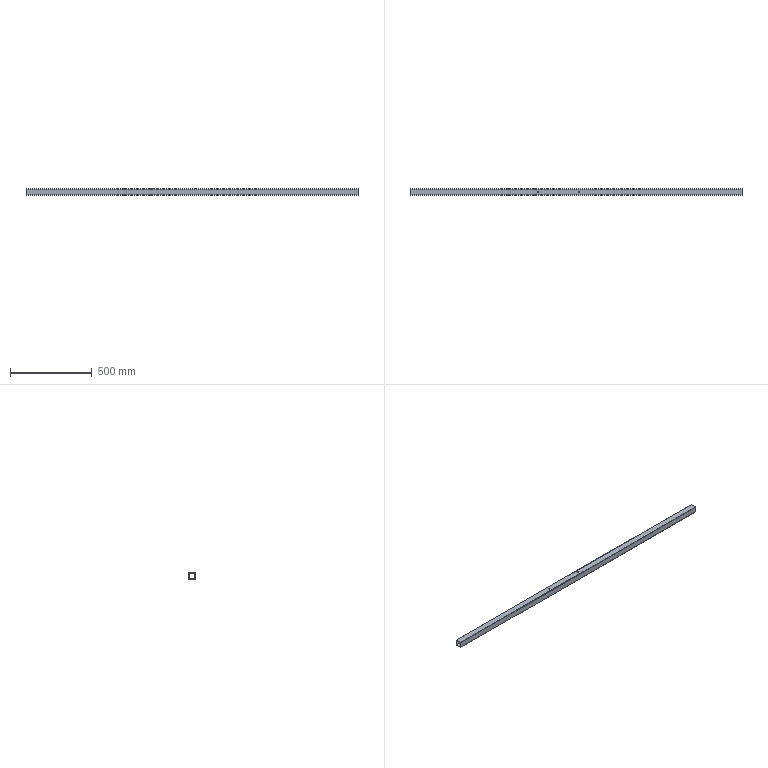Part | NX | features BREP 1 | 1 solid | 18 faces | box 2032 x 38.1 x 38.1 mm | volume 548857 mm3 | plane 10 | cylinder 8 | commonest cylinder face diameters 3.175 x4 5.842 x4
STEP:
#1=CARTESIAN_POINT('',(-1016.,19.05,-17.462));
#2=VERTEX_POINT('',#1);
#3=CARTESIAN_POINT('',(-1016.,19.05,17.462));
#4=VERTEX_POINT('',#3);
#5=CARTESIAN_POINT('',(-1016.,19.05,-17.462));
#6=DIRECTION('',(0.,0.,1.));
#7=VECTOR('',#6,1000.);
#8=LINE('',#5,#7);
#9=EDGE_CURVE('',#2,#4,#8,.T.);
#10=ORIENTED_EDGE('',*,*,#9,.F.);
#11=CARTESIAN_POINT('',(-1016.,17.462,-19.05));
#12=VERTEX_POINT('',#11);
#13=CARTESIAN_POINT('',(-1016.,17.462,-17.462));
#14=DIRECTION('',(-1.,0.,0.));
#15=DIRECTION('',(0.,1.,0.));
#16=AXIS2_PLACEMENT_3D('',#13,#14,#15);
#17=CIRCLE('',#16,1.587);
#18=EDGE_CURVE('',#2,#12,#17,.T.);
#19=ORIENTED_EDGE('',*,*,#18,.T.);
#20=CARTESIAN_POINT('',(-1016.,-17.462,-19.05));
#21=VERTEX_POINT('',#20);
#22=CARTESIAN_POINT('',(-1016.,-17.462,-19.05));
#23=DIRECTION('',(0.,1.,0.));
#24=VECTOR('',#23,1000.);
#25=LINE('',#22,#24);
#26=EDGE_CURVE('',#21,#12,#25,.T.);
#27=ORIENTED_EDGE('',*,*,#26,.F.);
#28=CARTESIAN_POINT('',(-1016.,-19.05,-17.462));
#29=VERTEX_POINT('',#28);
#30=CARTESIAN_POINT('',(-1016.,-17.462,-17.462));
#31=DIRECTION('',(-1.,0.,0.));
#32=DIRECTION('',(0.,0.,-1.));
#33=AXIS2_PLACEMENT_3D('',#30,#31,#32);
#34=CIRCLE('',#33,1.587);
#35=EDGE_CURVE('',#21,#29,#34,.T.);
#36=ORIENTED_EDGE('',*,*,#35,.T.);
#37=CARTESIAN_POINT('',(-1016.,-19.05,17.462));
#38=VERTEX_POINT('',#37);
#39=CARTESIAN_POINT('',(-1016.,-19.05,17.462));
#40=DIRECTION('',(0.,0.,-1.));
#41=VECTOR('',#40,1000.);
#42=LINE('',#39,#41);
#43=EDGE_CURVE('',#38,#29,#42,.T.);
#44=ORIENTED_EDGE('',*,*,#43,.F.);
#45=CARTESIAN_POINT('',(-1016.,-17.462,19.05));
#46=VERTEX_POINT('',#45);
#47=CARTESIAN_POINT('',(-1016.,-17.462,17.462));
#48=DIRECTION('',(-1.,0.,0.));
#49=DIRECTION('',(0.,-1.,0.));
#50=AXIS2_PLACEMENT_3D('',#47,#48,#49);
#51=CIRCLE('',#50,1.587);
#52=EDGE_CURVE('',#38,#46,#51,.T.);
#53=ORIENTED_EDGE('',*,*,#52,.T.);
#54=CARTESIAN_POINT('',(-1016.,17.462,19.05));
#55=VERTEX_POINT('',#54);
#56=CARTESIAN_POINT('',(-1016.,17.462,19.05));
#57=DIRECTION('',(0.,-1.,0.));
#58=VECTOR('',#57,1000.);
#59=LINE('',#56,#58);
#60=EDGE_CURVE('',#55,#46,#59,.T.);
#61=ORIENTED_EDGE('',*,*,#60,.F.);
#62=CARTESIAN_POINT('',(-1016.,17.462,17.462));
#63=DIRECTION('',(-1.,0.,0.));
#64=DIRECTION('',(0.,0.,1.));
#65=AXIS2_PLACEMENT_3D('',#62,#63,#64);
#66=CIRCLE('',#65,1.587);
#67=EDGE_CURVE('',#55,#4,#66,.T.);
#68=ORIENTED_EDGE('',*,*,#67,.T.);
#69=EDGE_LOOP('',(#10,#19,#27,#36,#44,#53,#61,#68));
#70=FACE_BOUND('',#69,.T.);
#71=CARTESIAN_POINT('',(-1016.,17.17,17.17));
#72=VERTEX_POINT('',#71);
#73=CARTESIAN_POINT('',(-1016.,17.17,-17.17));
#74=VERTEX_POINT('',#73);
#75=CARTESIAN_POINT('',(-1016.,17.17,17.17));
#76=DIRECTION('',(0.,0.,-1.));
#77=VECTOR('',#76,1000.);
#78=LINE('',#75,#77);
#79=EDGE_CURVE('',#72,#74,#78,.T.);
#80=ORIENTED_EDGE('',*,*,#79,.F.);
#81=CARTESIAN_POINT('',(-1016.,-17.17,17.17));
#82=VERTEX_POINT('',#81);
#83=CARTESIAN_POINT('',(-1016.,-17.17,17.17));
#84=DIRECTION('',(0.,1.,0.));
#85=VECTOR('',#84,1000.);
#86=LINE('',#83,#85);
#87=EDGE_CURVE('',#82,#72,#86,.T.);
#88=ORIENTED_EDGE('',*,*,#87,.F.);
#89=CARTESIAN_POINT('',(-1016.,-17.17,-17.17));
#90=VERTEX_POINT('',#89);
#91=CARTESIAN_POINT('',(-1016.,-17.17,-17.17));
#92=DIRECTION('',(0.,0.,1.));
#93=VECTOR('',#92,1000.);
#94=LINE('',#91,#93);
#95=EDGE_CURVE('',#90,#82,#94,.T.);
#96=ORIENTED_EDGE('',*,*,#95,.F.);
#97=CARTESIAN_POINT('',(-1016.,17.17,-17.17));
#98=DIRECTION('',(0.,-1.,0.));
#99=VECTOR('',#98,1000.);
#100=LINE('',#97,#99);
#101=EDGE_CURVE('',#74,#90,#100,.T.);
#102=ORIENTED_EDGE('',*,*,#101,.F.);
#103=EDGE_LOOP('',(#80,#88,#96,#102));
#104=FACE_BOUND('',#103,.T.);
#105=CARTESIAN_POINT('',(-1016.,0.,0.));
#106=DIRECTION('',(1.,0.,0.));
#107=DIRECTION('',(0.,1.,0.));
#108=AXIS2_PLACEMENT_3D('',#105,#106,#107);
#109=PLANE('',#108);
#110=ADVANCED_FACE('',(#70,#104),#109,.F.);
#111=CARTESIAN_POINT('',(1016.,-17.17,-17.17));
#112=VERTEX_POINT('',#111);
#113=CARTESIAN_POINT('',(-1016.,-17.17,-17.17));
#114=DIRECTION('',(1.,0.,0.));
#115=VECTOR('',#114,1000.);
#116=LINE('',#113,#115);
#117=EDGE_CURVE('',#90,#112,#116,.T.);
#118=ORIENTED_EDGE('',*,*,#117,.T.);
#119=CARTESIAN_POINT('',(1016.,17.17,-17.17));
#120=VERTEX_POINT('',#119);
#121=CARTESIAN_POINT('',(1016.,17.17,-17.17));
#122=DIRECTION('',(0.,-1.,0.));
#123=VECTOR('',#122,1000.);
#124=LINE('',#121,#123);
#125=EDGE_CURVE('',#120,#112,#124,.T.);
#126=ORIENTED_EDGE('',*,*,#125,.F.);
#127=CARTESIAN_POINT('',(-1016.,17.17,-17.17));
#128=DIRECTION('',(1.,0.,0.));
#129=VECTOR('',#128,1000.);
#130=LINE('',#127,#129);
#131=EDGE_CURVE('',#74,#120,#130,.T.);
#132=ORIENTED_EDGE('',*,*,#131,.F.);
#133=ORIENTED_EDGE('',*,*,#101,.T.);
#134=EDGE_LOOP('',(#118,#126,#132,#133));
#135=FACE_BOUND('',#134,.T.);
#136=CARTESIAN_POINT('',(-1016.,17.17,-17.17));
#137=DIRECTION('',(0.,0.,1.));
#138=DIRECTION('',(1.,0.,0.));
#139=AXIS2_PLACEMENT_3D('',#136,#137,#138);
#140=PLANE('',#139);
#141=ADVANCED_FACE('',(#135),#140,.T.);
#142=ORIENTED_EDGE('',*,*,#131,.T.);
#143=CARTESIAN_POINT('',(1016.,17.17,17.17));
#144=VERTEX_POINT('',#143);
#145=CARTESIAN_POINT('',(1016.,17.17,17.17));
#146=DIRECTION('',(0.,0.,-1.));
#147=VECTOR('',#146,1000.);
#148=LINE('',#145,#147);
#149=EDGE_CURVE('',#144,#120,#148,.T.);
#150=ORIENTED_EDGE('',*,*,#149,.F.);
#151=CARTESIAN_POINT('',(-1016.,17.17,17.17));
#152=DIRECTION('',(1.,0.,0.));
#153=VECTOR('',#152,1000.);
#154=LINE('',#151,#153);
#155=EDGE_CURVE('',#72,#144,#154,.T.);
#156=ORIENTED_EDGE('',*,*,#155,.F.);
#157=ORIENTED_EDGE('',*,*,#79,.T.);
#158=EDGE_LOOP('',(#142,#150,#156,#157));
#159=FACE_BOUND('',#158,.T.);
#160=CARTESIAN_POINT('',(-1016.,17.17,17.17));
#161=DIRECTION('',(0.,-1.,0.));
#162=DIRECTION('',(0.,0.,-1.));
#163=AXIS2_PLACEMENT_3D('',#160,#161,#162);
#164=PLANE('',#163);
#165=ADVANCED_FACE('',(#159),#164,.T.);
#166=ORIENTED_EDGE('',*,*,#155,.T.);
#167=CARTESIAN_POINT('',(1016.,-17.17,17.17));
#168=VERTEX_POINT('',#167);
#169=CARTESIAN_POINT('',(1016.,-17.17,17.17));
#170=DIRECTION('',(0.,1.,0.));
#171=VECTOR('',#170,1000.);
#172=LINE('',#169,#171);
#173=EDGE_CURVE('',#168,#144,#172,.T.);
#174=ORIENTED_EDGE('',*,*,#173,.F.);
#175=CARTESIAN_POINT('',(-1016.,-17.17,17.17));
#176=DIRECTION('',(1.,0.,0.));
#177=VECTOR('',#176,1000.);
#178=LINE('',#175,#177);
#179=EDGE_CURVE('',#82,#168,#178,.T.);
#180=ORIENTED_EDGE('',*,*,#179,.F.);
#181=ORIENTED_EDGE('',*,*,#87,.T.);
#182=EDGE_LOOP('',(#166,#174,#180,#181));
#183=FACE_BOUND('',#182,.T.);
#184=CARTESIAN_POINT('',(17.907,0.,17.17));
#185=VERTEX_POINT('',#184);
#186=CARTESIAN_POINT('',(23.749,0.,17.17));
#187=VERTEX_POINT('',#186);
#188=CARTESIAN_POINT('',(20.828,0.,17.17));
#189=DIRECTION('',(0.,0.,1.));
#190=DIRECTION('',(-1.,0.,0.));
#191=AXIS2_PLACEMENT_3D('',#188,#189,#190);
#192=CIRCLE('',#191,2.921);
#193=EDGE_CURVE('',#185,#187,#192,.T.);
#194=ORIENTED_EDGE('',*,*,#193,.T.);
#195=CARTESIAN_POINT('',(20.828,0.,17.17));
#196=DIRECTION('',(0.,0.,1.));
#197=DIRECTION('',(1.,0.,0.));
#198=AXIS2_PLACEMENT_3D('',#195,#196,#197);
#199=CIRCLE('',#198,2.921);
#200=EDGE_CURVE('',#187,#185,#199,.T.);
#201=ORIENTED_EDGE('',*,*,#200,.T.);
#202=EDGE_LOOP('',(#194,#201));
#203=FACE_BOUND('',#202,.T.);
#204=CARTESIAN_POINT('',(-233.553,0.,17.17));
#205=VERTEX_POINT('',#204);
#206=CARTESIAN_POINT('',(-227.711,0.,17.17));
#207=VERTEX_POINT('',#206);
#208=CARTESIAN_POINT('',(-230.632,0.,17.17));
#209=DIRECTION('',(0.,0.,1.));
#210=DIRECTION('',(-1.,0.,0.));
#211=AXIS2_PLACEMENT_3D('',#208,#209,#210);
#212=CIRCLE('',#211,2.921);
#213=EDGE_CURVE('',#205,#207,#212,.T.);
#214=ORIENTED_EDGE('',*,*,#213,.T.);
#215=CARTESIAN_POINT('',(-230.632,0.,17.17));
#216=DIRECTION('',(0.,0.,1.));
#217=DIRECTION('',(1.,0.,0.));
#218=AXIS2_PLACEMENT_3D('',#215,#216,#217);
#219=CIRCLE('',#218,2.921);
#220=EDGE_CURVE('',#207,#205,#219,.T.);
#221=ORIENTED_EDGE('',*,*,#220,.T.);
#222=EDGE_LOOP('',(#214,#221));
#223=FACE_BOUND('',#222,.T.);
#224=CARTESIAN_POINT('',(-1016.,-17.17,17.17));
#225=DIRECTION('',(0.,0.,-1.));
#226=DIRECTION('',(0.,-1.,0.));
#227=AXIS2_PLACEMENT_3D('',#224,#225,#226);
#228=PLANE('',#227);
#229=ADVANCED_FACE('',(#183,#203,#223),#228,.T.);
#230=ORIENTED_EDGE('',*,*,#179,.T.);
#231=CARTESIAN_POINT('',(1016.,-17.17,-17.17));
#232=DIRECTION('',(0.,0.,1.));
#233=VECTOR('',#232,1000.);
#234=LINE('',#231,#233);
#235=EDGE_CURVE('',#112,#168,#234,.T.);
#236=ORIENTED_EDGE('',*,*,#235,.F.);
#237=ORIENTED_EDGE('',*,*,#117,.F.);
#238=ORIENTED_EDGE('',*,*,#95,.T.);
#239=EDGE_LOOP('',(#230,#236,#237,#238));
#240=FACE_BOUND('',#239,.T.);
#241=CARTESIAN_POINT('',(-1016.,-17.17,-17.17));
#242=DIRECTION('',(0.,1.,0.));
#243=DIRECTION('',(1.,0.,0.));
#244=AXIS2_PLACEMENT_3D('',#241,#242,#243);
#245=PLANE('',#244);
#246=ADVANCED_FACE('',(#240),#245,.T.);
#247=CARTESIAN_POINT('',(1016.,17.462,19.05));
#248=VERTEX_POINT('',#247);
#249=CARTESIAN_POINT('',(1016.,-17.462,19.05));
#250=VERTEX_POINT('',#249);
#251=CARTESIAN_POINT('',(1016.,17.462,19.05));
#252=DIRECTION('',(0.,-1.,0.));
#253=VECTOR('',#252,1000.);
#254=LINE('',#251,#253);
#255=EDGE_CURVE('',#248,#250,#254,.T.);
#256=ORIENTED_EDGE('',*,*,#255,.T.);
#257=CARTESIAN_POINT('',(1016.,-19.05,17.462));
#258=VERTEX_POINT('',#257);
#259=CARTESIAN_POINT('',(1016.,-17.462,17.462));
#260=DIRECTION('',(1.,0.,0.));
#261=DIRECTION('',(0.,0.,1.));
#262=AXIS2_PLACEMENT_3D('',#259,#260,#261);
#263=CIRCLE('',#262,1.587);
#264=EDGE_CURVE('',#250,#258,#263,.T.);
#265=ORIENTED_EDGE('',*,*,#264,.T.);
#266=CARTESIAN_POINT('',(1016.,-19.05,-17.462));
#267=VERTEX_POINT('',#266);
#268=CARTESIAN_POINT('',(1016.,-19.05,17.462));
#269=DIRECTION('',(0.,0.,-1.));
#270=VECTOR('',#269,1000.);
#271=LINE('',#268,#270);
#272=EDGE_CURVE('',#258,#267,#271,.T.);
#273=ORIENTED_EDGE('',*,*,#272,.T.);
#274=CARTESIAN_POINT('',(1016.,-17.462,-19.05));
#275=VERTEX_POINT('',#274);
#276=CARTESIAN_POINT('',(1016.,-17.462,-17.462));
#277=DIRECTION('',(1.,0.,0.));
#278=DIRECTION('',(0.,-1.,0.));
#279=AXIS2_PLACEMENT_3D('',#276,#277,#278);
#280=CIRCLE('',#279,1.587);
#281=EDGE_CURVE('',#267,#275,#280,.T.);
#282=ORIENTED_EDGE('',*,*,#281,.T.);
#283=CARTESIAN_POINT('',(1016.,17.462,-19.05));
#284=VERTEX_POINT('',#283);
#285=CARTESIAN_POINT('',(1016.,-17.462,-19.05));
#286=DIRECTION('',(0.,1.,0.));
#287=VECTOR('',#286,1000.);
#288=LINE('',#285,#287);
#289=EDGE_CURVE('',#275,#284,#288,.T.);
#290=ORIENTED_EDGE('',*,*,#289,.T.);
#291=CARTESIAN_POINT('',(1016.,19.05,-17.462));
#292=VERTEX_POINT('',#291);
#293=CARTESIAN_POINT('',(1016.,17.462,-17.462));
#294=DIRECTION('',(1.,0.,0.));
#295=DIRECTION('',(0.,0.,-1.));
#296=AXIS2_PLACEMENT_3D('',#293,#294,#295);
#297=CIRCLE('',#296,1.587);
#298=EDGE_CURVE('',#284,#292,#297,.T.);
#299=ORIENTED_EDGE('',*,*,#298,.T.);
#300=CARTESIAN_POINT('',(1016.,19.05,17.462));
#301=VERTEX_POINT('',#300);
#302=CARTESIAN_POINT('',(1016.,19.05,-17.462));
#303=DIRECTION('',(0.,0.,1.));
#304=VECTOR('',#303,1000.);
#305=LINE('',#302,#304);
#306=EDGE_CURVE('',#292,#301,#305,.T.);
#307=ORIENTED_EDGE('',*,*,#306,.T.);
#308=CARTESIAN_POINT('',(1016.,17.462,17.462));
#309=DIRECTION('',(1.,0.,0.));
#310=DIRECTION('',(0.,1.,0.));
#311=AXIS2_PLACEMENT_3D('',#308,#309,#310);
#312=CIRCLE('',#311,1.587);
#313=EDGE_CURVE('',#301,#248,#312,.T.);
#314=ORIENTED_EDGE('',*,*,#313,.T.);
#315=EDGE_LOOP('',(#256,#265,#273,#282,#290,#299,#307,#314));
#316=FACE_BOUND('',#315,.T.);
#317=ORIENTED_EDGE('',*,*,#235,.T.);
#318=ORIENTED_EDGE('',*,*,#173,.T.);
#319=ORIENTED_EDGE('',*,*,#149,.T.);
#320=ORIENTED_EDGE('',*,*,#125,.T.);
#321=EDGE_LOOP('',(#317,#318,#319,#320));
#322=FACE_BOUND('',#321,.T.);
#323=CARTESIAN_POINT('',(1016.,0.,0.));
#324=DIRECTION('',(1.,0.,0.));
#325=DIRECTION('',(0.,1.,0.));
#326=AXIS2_PLACEMENT_3D('',#323,#324,#325);
#327=PLANE('',#326);
#328=ADVANCED_FACE('',(#316,#322),#327,.T.);
#329=ORIENTED_EDGE('',*,*,#313,.F.);
#330=CARTESIAN_POINT('',(1016.,19.05,17.462));
#331=DIRECTION('',(-1.,0.,0.));
#332=VECTOR('',#331,1000.);
#333=LINE('',#330,#332);
#334=EDGE_CURVE('',#301,#4,#333,.T.);
#335=ORIENTED_EDGE('',*,*,#334,.T.);
#336=ORIENTED_EDGE('',*,*,#67,.F.);
#337=CARTESIAN_POINT('',(1016.,17.462,19.05));
#338=DIRECTION('',(-1.,0.,0.));
#339=VECTOR('',#338,1000.);
#340=LINE('',#337,#339);
#341=EDGE_CURVE('',#248,#55,#340,.T.);
#342=ORIENTED_EDGE('',*,*,#341,.F.);
#343=EDGE_LOOP('',(#329,#335,#336,#342));
#344=FACE_BOUND('',#343,.T.);
#345=CARTESIAN_POINT('',(1019.181,17.462,17.462));
#346=DIRECTION('',(-1.,0.,0.));
#347=DIRECTION('',(0.,0.,1.));
#348=AXIS2_PLACEMENT_3D('',#345,#346,#347);
#349=CYLINDRICAL_SURFACE('',#348,1.587);
#350=ADVANCED_FACE('',(#344),#349,.T.);
#351=ORIENTED_EDGE('',*,*,#60,.T.);
#352=CARTESIAN_POINT('',(1016.,-17.462,19.05));
#353=DIRECTION('',(-1.,0.,0.));
#354=VECTOR('',#353,1000.);
#355=LINE('',#352,#354);
#356=EDGE_CURVE('',#250,#46,#355,.T.);
#357=ORIENTED_EDGE('',*,*,#356,.F.);
#358=ORIENTED_EDGE('',*,*,#255,.F.);
#359=ORIENTED_EDGE('',*,*,#341,.T.);
#360=EDGE_LOOP('',(#351,#357,#358,#359));
#361=FACE_BOUND('',#360,.T.);
#362=CARTESIAN_POINT('',(17.907,0.,19.05));
#363=VERTEX_POINT('',#362);
#364=CARTESIAN_POINT('',(23.749,0.,19.05));
#365=VERTEX_POINT('',#364);
#366=CARTESIAN_POINT('',(20.828,0.,19.05));
#367=DIRECTION('',(0.,0.,1.));
#368=DIRECTION('',(-1.,0.,0.));
#369=AXIS2_PLACEMENT_3D('',#366,#367,#368);
#370=CIRCLE('',#369,2.921);
#371=EDGE_CURVE('',#363,#365,#370,.T.);
#372=ORIENTED_EDGE('',*,*,#371,.F.);
#373=CARTESIAN_POINT('',(20.828,0.,19.05));
#374=DIRECTION('',(0.,0.,1.));
#375=DIRECTION('',(1.,0.,0.));
#376=AXIS2_PLACEMENT_3D('',#373,#374,#375);
#377=CIRCLE('',#376,2.921);
#378=EDGE_CURVE('',#365,#363,#377,.T.);
#379=ORIENTED_EDGE('',*,*,#378,.F.);
#380=EDGE_LOOP('',(#372,#379));
#381=FACE_BOUND('',#380,.T.);
#382=CARTESIAN_POINT('',(-233.553,0.,19.05));
#383=VERTEX_POINT('',#382);
#384=CARTESIAN_POINT('',(-227.711,0.,19.05));
#385=VERTEX_POINT('',#384);
#386=CARTESIAN_POINT('',(-230.632,0.,19.05));
#387=DIRECTION('',(0.,0.,1.));
#388=DIRECTION('',(-1.,0.,0.));
#389=AXIS2_PLACEMENT_3D('',#386,#387,#388);
#390=CIRCLE('',#389,2.921);
#391=EDGE_CURVE('',#383,#385,#390,.T.);
#392=ORIENTED_EDGE('',*,*,#391,.F.);
#393=CARTESIAN_POINT('',(-230.632,0.,19.05));
#394=DIRECTION('',(0.,0.,1.));
#395=DIRECTION('',(1.,0.,0.));
#396=AXIS2_PLACEMENT_3D('',#393,#394,#395);
#397=CIRCLE('',#396,2.921);
#398=EDGE_CURVE('',#385,#383,#397,.T.);
#399=ORIENTED_EDGE('',*,*,#398,.F.);
#400=EDGE_LOOP('',(#392,#399));
#401=FACE_BOUND('',#400,.T.);
#402=CARTESIAN_POINT('',(-1016.,19.05,19.05));
#403=DIRECTION('',(0.,0.,1.));
#404=DIRECTION('',(1.,0.,0.));
#405=AXIS2_PLACEMENT_3D('',#402,#403,#404);
#406=PLANE('',#405);
#407=ADVANCED_FACE('',(#361,#381,#401),#406,.T.);
#408=ORIENTED_EDGE('',*,*,#264,.F.);
#409=ORIENTED_EDGE('',*,*,#356,.T.);
#410=ORIENTED_EDGE('',*,*,#52,.F.);
#411=CARTESIAN_POINT('',(1016.,-19.05,17.462));
#412=DIRECTION('',(-1.,0.,0.));
#413=VECTOR('',#412,1000.);
#414=LINE('',#411,#413);
#415=EDGE_CURVE('',#258,#38,#414,.T.);
#416=ORIENTED_EDGE('',*,*,#415,.F.);
#417=EDGE_LOOP('',(#408,#409,#410,#416));
#418=FACE_BOUND('',#417,.T.);
#419=CARTESIAN_POINT('',(1019.181,-17.462,17.462));
#420=DIRECTION('',(-1.,0.,0.));
#421=DIRECTION('',(0.,-1.,0.));
#422=AXIS2_PLACEMENT_3D('',#419,#420,#421);
#423=CYLINDRICAL_SURFACE('',#422,1.587);
#424=ADVANCED_FACE('',(#418),#423,.T.);
#425=ORIENTED_EDGE('',*,*,#43,.T.);
#426=CARTESIAN_POINT('',(1016.,-19.05,-17.462));
#427=DIRECTION('',(-1.,0.,0.));
#428=VECTOR('',#427,1000.);
#429=LINE('',#426,#428);
#430=EDGE_CURVE('',#267,#29,#429,.T.);
#431=ORIENTED_EDGE('',*,*,#430,.F.);
#432=ORIENTED_EDGE('',*,*,#272,.F.);
#433=ORIENTED_EDGE('',*,*,#415,.T.);
#434=EDGE_LOOP('',(#425,#431,#432,#433));
#435=FACE_BOUND('',#434,.T.);
#436=CARTESIAN_POINT('',(-1016.,-19.05,19.05));
#437=DIRECTION('',(0.,-1.,0.));
#438=DIRECTION('',(0.,0.,-1.));
#439=AXIS2_PLACEMENT_3D('',#436,#437,#438);
#440=PLANE('',#439);
#441=ADVANCED_FACE('',(#435),#440,.T.);
#442=ORIENTED_EDGE('',*,*,#281,.F.);
#443=ORIENTED_EDGE('',*,*,#430,.T.);
#444=ORIENTED_EDGE('',*,*,#35,.F.);
#445=CARTESIAN_POINT('',(1016.,-17.462,-19.05));
#446=DIRECTION('',(-1.,0.,0.));
#447=VECTOR('',#446,1000.);
#448=LINE('',#445,#447);
#449=EDGE_CURVE('',#275,#21,#448,.T.);
#450=ORIENTED_EDGE('',*,*,#449,.F.);
#451=EDGE_LOOP('',(#442,#443,#444,#450));
#452=FACE_BOUND('',#451,.T.);
#453=CARTESIAN_POINT('',(1019.181,-17.462,-17.462));
#454=DIRECTION('',(-1.,0.,0.));
#455=DIRECTION('',(0.,0.,-1.));
#456=AXIS2_PLACEMENT_3D('',#453,#454,#455);
#457=CYLINDRICAL_SURFACE('',#456,1.587);
#458=ADVANCED_FACE('',(#452),#457,.T.);
#459=ORIENTED_EDGE('',*,*,#289,.F.);
#460=ORIENTED_EDGE('',*,*,#449,.T.);
#461=ORIENTED_EDGE('',*,*,#26,.T.);
#462=CARTESIAN_POINT('',(1016.,17.462,-19.05));
#463=DIRECTION('',(-1.,0.,0.));
#464=VECTOR('',#463,1000.);
#465=LINE('',#462,#464);
#466=EDGE_CURVE('',#284,#12,#465,.T.);
#467=ORIENTED_EDGE('',*,*,#466,.F.);
#468=EDGE_LOOP('',(#459,#460,#461,#467));
#469=FACE_BOUND('',#468,.T.);
#470=CARTESIAN_POINT('',(-1016.,-19.05,-19.05));
#471=DIRECTION('',(0.,0.,-1.));
#472=DIRECTION('',(0.,-1.,0.));
#473=AXIS2_PLACEMENT_3D('',#470,#471,#472);
#474=PLANE('',#473);
#475=ADVANCED_FACE('',(#469),#474,.T.);
#476=ORIENTED_EDGE('',*,*,#298,.F.);
#477=ORIENTED_EDGE('',*,*,#466,.T.);
#478=ORIENTED_EDGE('',*,*,#18,.F.);
#479=CARTESIAN_POINT('',(1016.,19.05,-17.462));
#480=DIRECTION('',(-1.,0.,0.));
#481=VECTOR('',#480,1000.);
#482=LINE('',#479,#481);
#483=EDGE_CURVE('',#292,#2,#482,.T.);
#484=ORIENTED_EDGE('',*,*,#483,.F.);
#485=EDGE_LOOP('',(#476,#477,#478,#484));
#486=FACE_BOUND('',#485,.T.);
#487=CARTESIAN_POINT('',(1019.181,17.462,-17.462));
#488=DIRECTION('',(-1.,0.,0.));
#489=DIRECTION('',(0.,1.,0.));
#490=AXIS2_PLACEMENT_3D('',#487,#488,#489);
#491=CYLINDRICAL_SURFACE('',#490,1.587);
#492=ADVANCED_FACE('',(#486),#491,.T.);
#493=ORIENTED_EDGE('',*,*,#306,.F.);
#494=ORIENTED_EDGE('',*,*,#483,.T.);
#495=ORIENTED_EDGE('',*,*,#9,.T.);
#496=ORIENTED_EDGE('',*,*,#334,.F.);
#497=EDGE_LOOP('',(#493,#494,#495,#496));
#498=FACE_BOUND('',#497,.T.);
#499=CARTESIAN_POINT('',(-1016.,19.05,-19.05));
#500=DIRECTION('',(0.,1.,0.));
#501=DIRECTION('',(1.,0.,0.));
#502=AXIS2_PLACEMENT_3D('',#499,#500,#501);
#503=PLANE('',#502);
#504=ADVANCED_FACE('',(#498),#503,.T.);
#505=CARTESIAN_POINT('',(17.907,0.,19.05));
#506=DIRECTION('',(0.,0.,-1.));
#507=VECTOR('',#506,1000.);
#508=LINE('',#505,#507);
#509=EDGE_CURVE('',#363,#185,#508,.T.);
#510=ORIENTED_EDGE('',*,*,#509,.T.);
#511=ORIENTED_EDGE('',*,*,#200,.F.);
#512=CARTESIAN_POINT('',(23.749,0.,19.05));
#513=DIRECTION('',(0.,0.,-1.));
#514=VECTOR('',#513,1000.);
#515=LINE('',#512,#514);
#516=EDGE_CURVE('',#365,#187,#515,.T.);
#517=ORIENTED_EDGE('',*,*,#516,.F.);
#518=ORIENTED_EDGE('',*,*,#378,.T.);
#519=EDGE_LOOP('',(#510,#511,#517,#518));
#520=FACE_BOUND('',#519,.T.);
#521=CARTESIAN_POINT('',(20.828,0.,19.05));
#522=DIRECTION('',(0.,0.,1.));
#523=DIRECTION('',(1.,0.,0.));
#524=AXIS2_PLACEMENT_3D('',#521,#522,#523);
#525=CYLINDRICAL_SURFACE('',#524,2.921);
#526=ADVANCED_FACE('',(#520),#525,.F.);
#527=ORIENTED_EDGE('',*,*,#516,.T.);
#528=ORIENTED_EDGE('',*,*,#193,.F.);
#529=ORIENTED_EDGE('',*,*,#509,.F.);
#530=ORIENTED_EDGE('',*,*,#371,.T.);
#531=EDGE_LOOP('',(#527,#528,#529,#530));
#532=FACE_BOUND('',#531,.T.);
#533=CARTESIAN_POINT('',(20.828,0.,19.05));
#534=DIRECTION('',(0.,0.,1.));
#535=DIRECTION('',(1.,0.,0.));
#536=AXIS2_PLACEMENT_3D('',#533,#534,#535);
#537=CYLINDRICAL_SURFACE('',#536,2.921);
#538=ADVANCED_FACE('',(#532),#537,.F.);
#539=CARTESIAN_POINT('',(-233.553,0.,19.05));
#540=DIRECTION('',(0.,0.,-1.));
#541=VECTOR('',#540,1000.);
#542=LINE('',#539,#541);
#543=EDGE_CURVE('',#383,#205,#542,.T.);
#544=ORIENTED_EDGE('',*,*,#543,.T.);
#545=ORIENTED_EDGE('',*,*,#220,.F.);
#546=CARTESIAN_POINT('',(-227.711,0.,19.05));
#547=DIRECTION('',(0.,0.,-1.));
#548=VECTOR('',#547,1000.);
#549=LINE('',#546,#548);
#550=EDGE_CURVE('',#385,#207,#549,.T.);
#551=ORIENTED_EDGE('',*,*,#550,.F.);
#552=ORIENTED_EDGE('',*,*,#398,.T.);
#553=EDGE_LOOP('',(#544,#545,#551,#552));
#554=FACE_BOUND('',#553,.T.);
#555=CARTESIAN_POINT('',(-230.632,0.,19.05));
#556=DIRECTION('',(0.,0.,1.));
#557=DIRECTION('',(1.,0.,0.));
#558=AXIS2_PLACEMENT_3D('',#555,#556,#557);
#559=CYLINDRICAL_SURFACE('',#558,2.921);
#560=ADVANCED_FACE('',(#554),#559,.F.);
#561=ORIENTED_EDGE('',*,*,#550,.T.);
#562=ORIENTED_EDGE('',*,*,#213,.F.);
#563=ORIENTED_EDGE('',*,*,#543,.F.);
#564=ORIENTED_EDGE('',*,*,#391,.T.);
#565=EDGE_LOOP('',(#561,#562,#563,#564));
#566=FACE_BOUND('',#565,.T.);
#567=CARTESIAN_POINT('',(-230.632,0.,19.05));
#568=DIRECTION('',(0.,0.,1.));
#569=DIRECTION('',(1.,0.,0.));
#570=AXIS2_PLACEMENT_3D('',#567,#568,#569);
#571=CYLINDRICAL_SURFACE('',#570,2.921);
#572=ADVANCED_FACE('',(#566),#571,.F.);
#573=CLOSED_SHELL('',(#110,#141,#165,#229,#246,#328,#350,#407,#424,#441,#458,#475,#492,#504,#526,#538,#560,#572));
#574=MANIFOLD_SOLID_BREP('',#573);
#575=(LENGTH_UNIT()NAMED_UNIT(*)SI_UNIT(.MILLI.,.METRE.));
#576=UNCERTAINTY_MEASURE_WITH_UNIT(LENGTH_MEASURE(0.00001),#575,'','');
#577=(NAMED_UNIT(*)PLANE_ANGLE_UNIT()SI_UNIT($,.RADIAN.));
#578=(NAMED_UNIT(*)SI_UNIT($,.STERADIAN.)SOLID_ANGLE_UNIT());
#579=(GEOMETRIC_REPRESENTATION_CONTEXT(3)GLOBAL_UNCERTAINTY_ASSIGNED_CONTEXT((#576))GLOBAL_UNIT_ASSIGNED_CONTEXT((#575,#577,#578))REPRESENTATION_CONTEXT('',''));
#580=ADVANCED_BREP_SHAPE_REPRESENTATION('',(#574),#579);